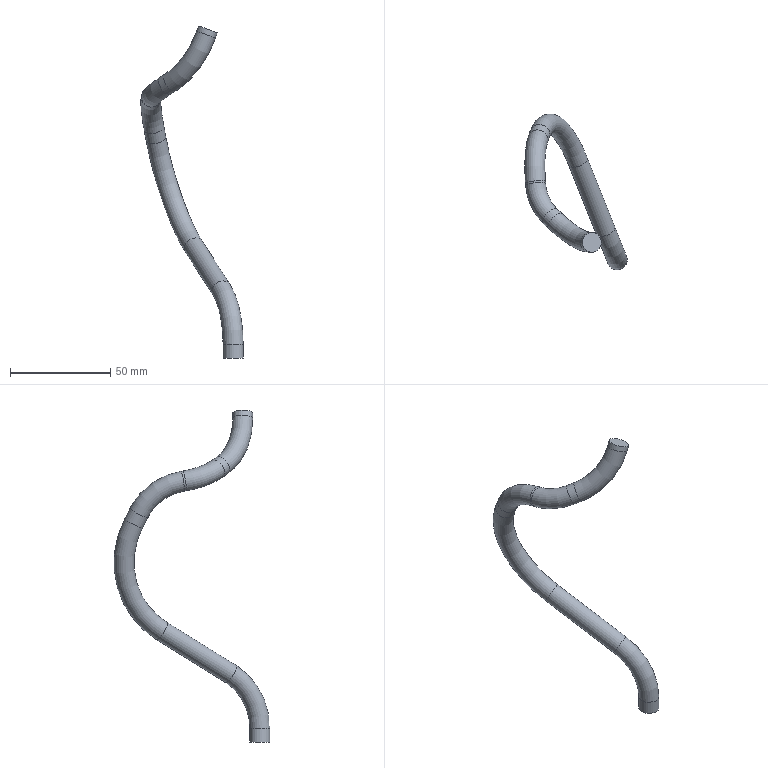Part | STEP file | DEWALT-DWE7294-B3-03 | 1 solid | 13 faces | box 51.027 x 77.706 x 165.503 mm | volume 18773 mm3 | cylinder 6 | torus 5 | plane 2 | commonest cylinder face diameters 10 x6
STEP:
#1=CARTESIAN_POINT('',(0.,0.,0.));
#2=DIRECTION('',(0.,0.,1.));
#3=DIRECTION('',(1.,0.,0.));
#4=AXIS2_PLACEMENT_3D('',#1,#2,#3);
#5=CARTESIAN_POINT('',(5.,0.,0.));
#6=VERTEX_POINT('',#5);
#7=CARTESIAN_POINT('',(0.,0.,0.));
#8=DIRECTION('',(0.,0.,-1.));
#9=DIRECTION('',(1.,0.,0.));
#10=AXIS2_PLACEMENT_3D('',#7,#8,#9);
#11=CIRCLE('',#10,5.);
#12=CARTESIAN_POINT('',(0.,0.,6.811));
#13=DIRECTION('',(0.,0.,-1.));
#14=DIRECTION('',(-1.,0.,0.));
#15=AXIS2_PLACEMENT_3D('',#12,#13,#14);
#16=CYLINDRICAL_SURFACE('',#15,5.);
#17=CARTESIAN_POINT('',(3.142,6.811));
#18=DIRECTION('',(1.,0.));
#19=VECTOR('',#18,1.);
#20=LINE('',#17,#19);
#21=(GEOMETRIC_REPRESENTATION_CONTEXT(2)PARAMETRIC_REPRESENTATION_CONTEXT()REPRESENTATION_CONTEXT('',''));
#22=DEFINITIONAL_REPRESENTATION('',(#20),#21);
#23=PCURVE('',#16,#22);
#24=CARTESIAN_POINT('',(0.,0.,0.));
#25=DIRECTION('',(0.,0.,-1.));
#26=DIRECTION('',(-1.,0.,0.));
#27=AXIS2_PLACEMENT_3D('',#24,#25,#26);
#28=PLANE('',#27);
#29=CARTESIAN_POINT('',(0.,0.));
#30=DIRECTION('',(-1.,0.));
#31=AXIS2_PLACEMENT_2D('',#29,#30);
#32=CIRCLE('',#31,5.);
#33=(GEOMETRIC_REPRESENTATION_CONTEXT(2)PARAMETRIC_REPRESENTATION_CONTEXT()REPRESENTATION_CONTEXT('',''));
#34=DEFINITIONAL_REPRESENTATION('',(#32),#33);
#35=PCURVE('',#28,#34);
#36=SURFACE_CURVE('',#11,(#23,#35),.PCURVE_S1.);
#37=EDGE_CURVE('',#6,#6,#36,.T.);
#38=ORIENTED_EDGE('',*,*,#37,.F.);
#39=CARTESIAN_POINT('',(5.,0.,6.811));
#40=VERTEX_POINT('',#39);
#41=CARTESIAN_POINT('',(5.,0.,6.811));
#42=CARTESIAN_POINT('',(5.,0.,0.));
#43=B_SPLINE_CURVE_WITH_KNOTS('',1,(#41,#42),.UNSPECIFIED.,.F.,.F.,(2,2),(0.,6.811),.PIECEWISE_BEZIER_KNOTS.);
#44=CARTESIAN_POINT('',(3.142,0.));
#45=DIRECTION('',(0.,1.));
#46=VECTOR('',#45,1.);
#47=LINE('',#44,#46);
#48=(GEOMETRIC_REPRESENTATION_CONTEXT(2)PARAMETRIC_REPRESENTATION_CONTEXT()REPRESENTATION_CONTEXT('',''));
#49=DEFINITIONAL_REPRESENTATION('',(#47),#48);
#50=PCURVE('',#16,#49);
#51=CARTESIAN_POINT('',(9.425,0.));
#52=DIRECTION('',(0.,1.));
#53=VECTOR('',#52,1.);
#54=LINE('',#51,#53);
#55=(GEOMETRIC_REPRESENTATION_CONTEXT(2)PARAMETRIC_REPRESENTATION_CONTEXT()REPRESENTATION_CONTEXT('',''));
#56=DEFINITIONAL_REPRESENTATION('',(#54),#55);
#57=PCURVE('',#16,#56);
#58=SEAM_CURVE('',#43,(#50,#57),.PCURVE_S1.);
#59=EDGE_CURVE('',#40,#6,#58,.T.);
#60=ORIENTED_EDGE('',*,*,#59,.F.);
#61=CARTESIAN_POINT('',(0.,0.,6.811));
#62=DIRECTION('',(0.,0.,-1.));
#63=DIRECTION('',(1.,0.,0.));
#64=AXIS2_PLACEMENT_3D('',#61,#62,#63);
#65=CIRCLE('',#64,5.);
#66=CARTESIAN_POINT('',(3.142,0.));
#67=DIRECTION('',(1.,0.));
#68=VECTOR('',#67,1.);
#69=LINE('',#66,#68);
#70=(GEOMETRIC_REPRESENTATION_CONTEXT(2)PARAMETRIC_REPRESENTATION_CONTEXT()REPRESENTATION_CONTEXT('',''));
#71=DEFINITIONAL_REPRESENTATION('',(#69),#70);
#72=PCURVE('',#16,#71);
#73=CARTESIAN_POINT('',(-11.672,29.262,6.811));
#74=DIRECTION('',(0.9288,0.3705,0.));
#75=DIRECTION('',(-0.3705,0.9288,0.));
#76=AXIS2_PLACEMENT_3D('',#73,#74,#75);
#77=TOROIDAL_SURFACE('',#76,31.504,5.);
#78=CARTESIAN_POINT('',(3.142,7.474));
#79=DIRECTION('',(0.,-1.));
#80=VECTOR('',#79,1.);
#81=LINE('',#78,#80);
#82=(GEOMETRIC_REPRESENTATION_CONTEXT(2)PARAMETRIC_REPRESENTATION_CONTEXT()REPRESENTATION_CONTEXT('',''));
#83=DEFINITIONAL_REPRESENTATION('',(#81),#82);
#84=PCURVE('',#77,#83);
#85=SURFACE_CURVE('',#65,(#72,#84),.PCURVE_S1.);
#86=EDGE_CURVE('',#40,#40,#85,.T.);
#87=ORIENTED_EDGE('',*,*,#86,.T.);
#88=ORIENTED_EDGE('',*,*,#59,.T.);
#89=EDGE_LOOP('',(#38,#60,#87,#88));
#90=FACE_BOUND('',#89,.T.);
#91=ADVANCED_FACE('',(#90),#16,.T.);
#92=ORIENTED_EDGE('',*,*,#86,.F.);
#93=CARTESIAN_POINT('',(-1.179,15.491,35.699));
#94=VERTEX_POINT('',#93);
#95=CARTESIAN_POINT('',(-1.179,15.491,35.699));
#96=CARTESIAN_POINT('',(0.706,10.765,32.761));
#97=CARTESIAN_POINT('',(2.341,6.666,28.785));
#98=CARTESIAN_POINT('',(3.641,3.406,23.952));
#99=CARTESIAN_POINT('',(4.542,1.149,18.496));
#100=CARTESIAN_POINT('',(5.,0.,12.687));
#101=CARTESIAN_POINT('',(5.,0.,6.811));
#102=(BOUNDED_CURVE()B_SPLINE_CURVE(6,(#95,#96,#97,#98,#99,#100,#101),.UNSPECIFIED.,.F.,.F.)B_SPLINE_CURVE_WITH_KNOTS((7,7),(2.094,3.142),.PIECEWISE_BEZIER_KNOTS.)CURVE()GEOMETRIC_REPRESENTATION_ITEM()RATIONAL_B_SPLINE_CURVE((1.014,1.005,0.9991,0.9973,0.9991,1.005,1.014))REPRESENTATION_ITEM(''));
#103=CARTESIAN_POINT('',(0.,7.474));
#104=DIRECTION('',(1.,0.));
#105=VECTOR('',#104,1.);
#106=LINE('',#103,#105);
#107=(GEOMETRIC_REPRESENTATION_CONTEXT(2)PARAMETRIC_REPRESENTATION_CONTEXT()REPRESENTATION_CONTEXT('',''));
#108=DEFINITIONAL_REPRESENTATION('',(#106),#107);
#109=PCURVE('',#77,#108);
#110=CARTESIAN_POINT('',(0.,1.191));
#111=DIRECTION('',(1.,0.));
#112=VECTOR('',#111,1.);
#113=LINE('',#110,#112);
#114=(GEOMETRIC_REPRESENTATION_CONTEXT(2)PARAMETRIC_REPRESENTATION_CONTEXT()REPRESENTATION_CONTEXT('',''));
#115=DEFINITIONAL_REPRESENTATION('',(#113),#114);
#116=PCURVE('',#77,#115);
#117=SEAM_CURVE('',#102,(#109,#116),.PCURVE_S1.);
#118=EDGE_CURVE('',#94,#40,#117,.T.);
#119=ORIENTED_EDGE('',*,*,#118,.F.);
#120=CARTESIAN_POINT('',(-5.836,14.631,34.094));
#121=DIRECTION('',(0.3209,-0.8044,-0.5));
#122=DIRECTION('',(0.9314,0.1721,0.3209));
#123=AXIS2_PLACEMENT_3D('',#120,#121,#122);
#124=CIRCLE('',#123,5.);
#125=CARTESIAN_POINT('',(2.094,7.474));
#126=DIRECTION('',(0.,-1.));
#127=VECTOR('',#126,1.);
#128=LINE('',#125,#127);
#129=(GEOMETRIC_REPRESENTATION_CONTEXT(2)PARAMETRIC_REPRESENTATION_CONTEXT()REPRESENTATION_CONTEXT('',''));
#130=DEFINITIONAL_REPRESENTATION('',(#128),#129);
#131=PCURVE('',#77,#130);
#132=CARTESIAN_POINT('',(-19.569,49.06,55.495));
#133=DIRECTION('',(0.3209,-0.8044,-0.5));
#134=DIRECTION('',(0.,0.5279,-0.8493));
#135=AXIS2_PLACEMENT_3D('',#132,#133,#134);
#136=CYLINDRICAL_SURFACE('',#135,5.);
#137=CARTESIAN_POINT('',(1.753,42.801));
#138=DIRECTION('',(1.,0.));
#139=VECTOR('',#138,1.);
#140=LINE('',#137,#139);
#141=(GEOMETRIC_REPRESENTATION_CONTEXT(2)PARAMETRIC_REPRESENTATION_CONTEXT()REPRESENTATION_CONTEXT('',''));
#142=DEFINITIONAL_REPRESENTATION('',(#140),#141);
#143=PCURVE('',#136,#142);
#144=SURFACE_CURVE('',#124,(#131,#143),.PCURVE_S1.);
#145=EDGE_CURVE('',#94,#94,#144,.T.);
#146=ORIENTED_EDGE('',*,*,#145,.T.);
#147=ORIENTED_EDGE('',*,*,#118,.T.);
#148=EDGE_LOOP('',(#92,#119,#146,#147));
#149=FACE_BOUND('',#148,.T.);
#150=ADVANCED_FACE('',(#149),#77,.T.);
#151=ORIENTED_EDGE('',*,*,#145,.F.);
#152=CARTESIAN_POINT('',(-14.913,49.92,57.099));
#153=VERTEX_POINT('',#152);
#154=CARTESIAN_POINT('',(-14.913,49.92,57.099));
#155=CARTESIAN_POINT('',(-1.179,15.491,35.699));
#156=B_SPLINE_CURVE_WITH_KNOTS('',1,(#154,#155),.UNSPECIFIED.,.F.,.F.,(2,2),(0.,42.801),.PIECEWISE_BEZIER_KNOTS.);
#157=CARTESIAN_POINT('',(1.753,0.));
#158=DIRECTION('',(0.,1.));
#159=VECTOR('',#158,1.);
#160=LINE('',#157,#159);
#161=(GEOMETRIC_REPRESENTATION_CONTEXT(2)PARAMETRIC_REPRESENTATION_CONTEXT()REPRESENTATION_CONTEXT('',''));
#162=DEFINITIONAL_REPRESENTATION('',(#160),#161);
#163=PCURVE('',#136,#162);
#164=CARTESIAN_POINT('',(8.037,0.));
#165=DIRECTION('',(0.,1.));
#166=VECTOR('',#165,1.);
#167=LINE('',#164,#166);
#168=(GEOMETRIC_REPRESENTATION_CONTEXT(2)PARAMETRIC_REPRESENTATION_CONTEXT()REPRESENTATION_CONTEXT('',''));
#169=DEFINITIONAL_REPRESENTATION('',(#167),#168);
#170=PCURVE('',#136,#169);
#171=SEAM_CURVE('',#156,(#163,#170),.PCURVE_S1.);
#172=EDGE_CURVE('',#153,#94,#171,.T.);
#173=ORIENTED_EDGE('',*,*,#172,.F.);
#174=CARTESIAN_POINT('',(-19.569,49.06,55.495));
#175=DIRECTION('',(0.3209,-0.8044,-0.5));
#176=DIRECTION('',(0.9314,0.1721,0.3209));
#177=AXIS2_PLACEMENT_3D('',#174,#175,#176);
#178=CIRCLE('',#177,5.);
#179=CARTESIAN_POINT('',(1.753,0.));
#180=DIRECTION('',(1.,0.));
#181=VECTOR('',#180,1.);
#182=LINE('',#179,#181);
#183=(GEOMETRIC_REPRESENTATION_CONTEXT(2)PARAMETRIC_REPRESENTATION_CONTEXT()REPRESENTATION_CONTEXT('',''));
#184=DEFINITIONAL_REPRESENTATION('',(#182),#183);
#185=PCURVE('',#136,#184);
#186=CARTESIAN_POINT('',(-25.022,24.287,91.849));
#187=DIRECTION('',(-0.9391,-0.2016,-0.2783));
#188=DIRECTION('',(-0.2841,0.,0.9588));
#189=AXIS2_PLACEMENT_3D('',#186,#187,#188);
#190=TOROIDAL_SURFACE('',#189,44.329,5.);
#191=CARTESIAN_POINT('',(2.534,4.66));
#192=DIRECTION('',(0.,-1.));
#193=VECTOR('',#192,1.);
#194=LINE('',#191,#193);
#195=(GEOMETRIC_REPRESENTATION_CONTEXT(2)PARAMETRIC_REPRESENTATION_CONTEXT()REPRESENTATION_CONTEXT('',''));
#196=DEFINITIONAL_REPRESENTATION('',(#194),#195);
#197=PCURVE('',#190,#196);
#198=SURFACE_CURVE('',#178,(#185,#197),.PCURVE_S1.);
#199=EDGE_CURVE('',#153,#153,#198,.T.);
#200=ORIENTED_EDGE('',*,*,#199,.T.);
#201=ORIENTED_EDGE('',*,*,#172,.T.);
#202=EDGE_LOOP('',(#151,#173,#200,#201));
#203=FACE_BOUND('',#202,.T.);
#204=ADVANCED_FACE('',(#203),#136,.T.);
#205=ORIENTED_EDGE('',*,*,#199,.F.);
#206=CARTESIAN_POINT('',(-33.669,63.584,110.499));
#207=VERTEX_POINT('',#206);
#208=CARTESIAN_POINT('',(-33.669,63.584,110.499));
#209=CARTESIAN_POINT('',(-31.912,68.461,101.037));
#210=CARTESIAN_POINT('',(-29.242,70.498,90.549));
#211=CARTESIAN_POINT('',(-25.886,69.431,79.995));
#212=CARTESIAN_POINT('',(-22.148,65.33,70.351));
#213=CARTESIAN_POINT('',(-18.374,58.599,62.494));
#214=CARTESIAN_POINT('',(-14.913,49.92,57.099));
#215=(BOUNDED_CURVE()B_SPLINE_CURVE(6,(#208,#209,#210,#211,#212,#213,#214),.UNSPECIFIED.,.F.,.F.)B_SPLINE_CURVE_WITH_KNOTS((7,7),(1.091,2.534),.PIECEWISE_BEZIER_KNOTS.)CURVE()GEOMETRIC_REPRESENTATION_ITEM()RATIONAL_B_SPLINE_CURVE((1.026,1.008,0.9982,0.9949,0.9982,1.008,1.026))REPRESENTATION_ITEM(''));
#216=CARTESIAN_POINT('',(0.,4.66));
#217=DIRECTION('',(1.,0.));
#218=VECTOR('',#217,1.);
#219=LINE('',#216,#218);
#220=(GEOMETRIC_REPRESENTATION_CONTEXT(2)PARAMETRIC_REPRESENTATION_CONTEXT()REPRESENTATION_CONTEXT('',''));
#221=DEFINITIONAL_REPRESENTATION('',(#219),#220);
#222=PCURVE('',#190,#221);
#223=CARTESIAN_POINT('',(0.,-1.623));
#224=DIRECTION('',(1.,0.));
#225=VECTOR('',#224,1.);
#226=LINE('',#223,#225);
#227=(GEOMETRIC_REPRESENTATION_CONTEXT(2)PARAMETRIC_REPRESENTATION_CONTEXT()REPRESENTATION_CONTEXT('',''));
#228=DEFINITIONAL_REPRESENTATION('',(#226),#227);
#229=PCURVE('',#190,#228);
#230=SEAM_CURVE('',#215,(#222,#229),.PCURVE_S1.);
#231=EDGE_CURVE('',#207,#153,#230,.T.);
#232=ORIENTED_EDGE('',*,*,#231,.F.);
#233=CARTESIAN_POINT('',(-38.437,62.805,109.213));
#234=DIRECTION('',(0.1628,0.452,-0.877));
#235=DIRECTION('',(0.9537,0.1558,0.2573));
#236=AXIS2_PLACEMENT_3D('',#233,#234,#235);
#237=CIRCLE('',#236,5.);
#238=CARTESIAN_POINT('',(1.091,4.66));
#239=DIRECTION('',(0.,-1.));
#240=VECTOR('',#239,1.);
#241=LINE('',#238,#240);
#242=(GEOMETRIC_REPRESENTATION_CONTEXT(2)PARAMETRIC_REPRESENTATION_CONTEXT()REPRESENTATION_CONTEXT('',''));
#243=DEFINITIONAL_REPRESENTATION('',(#241),#242);
#244=PCURVE('',#190,#243);
#245=CARTESIAN_POINT('',(-39.385,60.173,114.32));
#246=DIRECTION('',(0.1628,0.452,-0.877));
#247=DIRECTION('',(0.,0.8889,0.4582));
#248=AXIS2_PLACEMENT_3D('',#245,#246,#247);
#249=CYLINDRICAL_SURFACE('',#248,5.);
#250=CARTESIAN_POINT('',(1.312,5.823));
#251=DIRECTION('',(1.,0.));
#252=VECTOR('',#251,1.);
#253=LINE('',#250,#252);
#254=(GEOMETRIC_REPRESENTATION_CONTEXT(2)PARAMETRIC_REPRESENTATION_CONTEXT()REPRESENTATION_CONTEXT('',''));
#255=DEFINITIONAL_REPRESENTATION('',(#253),#254);
#256=PCURVE('',#249,#255);
#257=SURFACE_CURVE('',#237,(#244,#256),.PCURVE_S1.);
#258=EDGE_CURVE('',#207,#207,#257,.T.);
#259=ORIENTED_EDGE('',*,*,#258,.T.);
#260=ORIENTED_EDGE('',*,*,#231,.T.);
#261=EDGE_LOOP('',(#205,#232,#259,#260));
#262=FACE_BOUND('',#261,.T.);
#263=ADVANCED_FACE('',(#262),#190,.T.);
#264=ORIENTED_EDGE('',*,*,#258,.F.);
#265=CARTESIAN_POINT('',(-34.617,60.952,115.606));
#266=VERTEX_POINT('',#265);
#267=CARTESIAN_POINT('',(-34.617,60.952,115.606));
#268=CARTESIAN_POINT('',(-33.669,63.584,110.499));
#269=B_SPLINE_CURVE_WITH_KNOTS('',1,(#267,#268),.UNSPECIFIED.,.F.,.F.,(2,2),(0.,5.823),.PIECEWISE_BEZIER_KNOTS.);
#270=CARTESIAN_POINT('',(1.312,0.));
#271=DIRECTION('',(0.,1.));
#272=VECTOR('',#271,1.);
#273=LINE('',#270,#272);
#274=(GEOMETRIC_REPRESENTATION_CONTEXT(2)PARAMETRIC_REPRESENTATION_CONTEXT()REPRESENTATION_CONTEXT('',''));
#275=DEFINITIONAL_REPRESENTATION('',(#273),#274);
#276=PCURVE('',#249,#275);
#277=CARTESIAN_POINT('',(7.595,0.));
#278=DIRECTION('',(0.,1.));
#279=VECTOR('',#278,1.);
#280=LINE('',#277,#279);
#281=(GEOMETRIC_REPRESENTATION_CONTEXT(2)PARAMETRIC_REPRESENTATION_CONTEXT()REPRESENTATION_CONTEXT('',''));
#282=DEFINITIONAL_REPRESENTATION('',(#280),#281);
#283=PCURVE('',#249,#282);
#284=SEAM_CURVE('',#269,(#276,#283),.PCURVE_S1.);
#285=EDGE_CURVE('',#266,#207,#284,.T.);
#286=ORIENTED_EDGE('',*,*,#285,.F.);
#287=CARTESIAN_POINT('',(-39.385,60.173,114.32));
#288=DIRECTION('',(0.1628,0.452,-0.877));
#289=DIRECTION('',(0.9537,0.1558,0.2573));
#290=AXIS2_PLACEMENT_3D('',#287,#288,#289);
#291=CIRCLE('',#290,5.);
#292=CARTESIAN_POINT('',(1.312,0.));
#293=DIRECTION('',(1.,0.));
#294=VECTOR('',#293,1.);
#295=LINE('',#292,#294);
#296=(GEOMETRIC_REPRESENTATION_CONTEXT(2)PARAMETRIC_REPRESENTATION_CONTEXT()REPRESENTATION_CONTEXT('',''));
#297=DEFINITIONAL_REPRESENTATION('',(#295),#296);
#298=PCURVE('',#249,#297);
#299=CARTESIAN_POINT('',(-33.388,34.461,102.18));
#300=DIRECTION('',(-0.9648,-0.113,-0.2373));
#301=DIRECTION('',(-0.2389,0.,0.9711));
#302=AXIS2_PLACEMENT_3D('',#299,#300,#301);
#303=TOROIDAL_SURFACE('',#302,29.059,5.);
#304=CARTESIAN_POINT('',(1.098,4.761));
#305=DIRECTION('',(0.,-1.));
#306=VECTOR('',#305,1.);
#307=LINE('',#304,#306);
#308=(GEOMETRIC_REPRESENTATION_CONTEXT(2)PARAMETRIC_REPRESENTATION_CONTEXT()REPRESENTATION_CONTEXT('',''));
#309=DEFINITIONAL_REPRESENTATION('',(#307),#308);
#310=PCURVE('',#303,#309);
#311=SURFACE_CURVE('',#291,(#298,#310),.PCURVE_S1.);
#312=EDGE_CURVE('',#266,#266,#311,.T.);
#313=ORIENTED_EDGE('',*,*,#312,.T.);
#314=ORIENTED_EDGE('',*,*,#285,.T.);
#315=EDGE_LOOP('',(#264,#286,#313,#314));
#316=FACE_BOUND('',#315,.T.);
#317=ADVANCED_FACE('',(#316),#249,.T.);
#318=ORIENTED_EDGE('',*,*,#312,.F.);
#319=CARTESIAN_POINT('',(-35.941,38.984,131.447));
#320=VERTEX_POINT('',#319);
#321=CARTESIAN_POINT('',(-35.941,38.984,131.447));
#322=CARTESIAN_POINT('',(-36.302,43.645,130.695));
#323=CARTESIAN_POINT('',(-36.429,48.139,129.073));
#324=CARTESIAN_POINT('',(-36.315,52.275,126.639));
#325=CARTESIAN_POINT('',(-35.962,55.881,123.49));
#326=CARTESIAN_POINT('',(-35.388,58.811,119.759));
#327=CARTESIAN_POINT('',(-34.617,60.952,115.606));
#328=(BOUNDED_CURVE()B_SPLINE_CURVE(6,(#321,#322,#323,#324,#325,#326,#327),.UNSPECIFIED.,.F.,.F.)B_SPLINE_CURVE_WITH_KNOTS((7,7),(0.1364,1.098),.PIECEWISE_BEZIER_KNOTS.)CURVE()GEOMETRIC_REPRESENTATION_ITEM()RATIONAL_B_SPLINE_CURVE((1.012,1.004,0.9992,0.9977,0.9992,1.004,1.012))REPRESENTATION_ITEM(''));
#329=CARTESIAN_POINT('',(0.,4.761));
#330=DIRECTION('',(1.,0.));
#331=VECTOR('',#330,1.);
#332=LINE('',#329,#331);
#333=(GEOMETRIC_REPRESENTATION_CONTEXT(2)PARAMETRIC_REPRESENTATION_CONTEXT()REPRESENTATION_CONTEXT('',''));
#334=DEFINITIONAL_REPRESENTATION('',(#332),#333);
#335=PCURVE('',#303,#334);
#336=CARTESIAN_POINT('',(0.,-1.522));
#337=DIRECTION('',(1.,0.));
#338=VECTOR('',#337,1.);
#339=LINE('',#336,#338);
#340=(GEOMETRIC_REPRESENTATION_CONTEXT(2)PARAMETRIC_REPRESENTATION_CONTEXT()REPRESENTATION_CONTEXT('',''));
#341=DEFINITIONAL_REPRESENTATION('',(#339),#340);
#342=PCURVE('',#303,#341);
#343=SEAM_CURVE('',#328,(#335,#342),.PCURVE_S1.);
#344=EDGE_CURVE('',#320,#266,#343,.T.);
#345=ORIENTED_EDGE('',*,*,#344,.F.);
#346=CARTESIAN_POINT('',(-40.698,38.387,130.029));
#347=DIRECTION('',(-0.0762,0.9844,-0.1588));
#348=DIRECTION('',(0.9515,0.1194,0.2836));
#349=AXIS2_PLACEMENT_3D('',#346,#347,#348);
#350=CIRCLE('',#349,5.);
#351=CARTESIAN_POINT('',(0.1364,4.761));
#352=DIRECTION('',(0.,-1.));
#353=VECTOR('',#352,1.);
#354=LINE('',#351,#353);
#355=(GEOMETRIC_REPRESENTATION_CONTEXT(2)PARAMETRIC_REPRESENTATION_CONTEXT()REPRESENTATION_CONTEXT('',''));
#356=DEFINITIONAL_REPRESENTATION('',(#354),#355);
#357=PCURVE('',#303,#356);
#358=CARTESIAN_POINT('',(-40.622,37.403,130.188));
#359=DIRECTION('',(-0.0762,0.9844,-0.1588));
#360=DIRECTION('',(0.,0.1593,0.9872));
#361=AXIS2_PLACEMENT_3D('',#358,#359,#360);
#362=CYLINDRICAL_SURFACE('',#361,5.);
#363=CARTESIAN_POINT('',(1.267,1.));
#364=DIRECTION('',(1.,0.));
#365=VECTOR('',#364,1.);
#366=LINE('',#363,#365);
#367=(GEOMETRIC_REPRESENTATION_CONTEXT(2)PARAMETRIC_REPRESENTATION_CONTEXT()REPRESENTATION_CONTEXT('',''));
#368=DEFINITIONAL_REPRESENTATION('',(#366),#367);
#369=PCURVE('',#362,#368);
#370=SURFACE_CURVE('',#350,(#357,#369),.PCURVE_S1.);
#371=EDGE_CURVE('',#320,#320,#370,.T.);
#372=ORIENTED_EDGE('',*,*,#371,.T.);
#373=ORIENTED_EDGE('',*,*,#344,.T.);
#374=EDGE_LOOP('',(#318,#345,#372,#373));
#375=FACE_BOUND('',#374,.T.);
#376=ADVANCED_FACE('',(#375),#303,.T.);
#377=ORIENTED_EDGE('',*,*,#371,.F.);
#378=CARTESIAN_POINT('',(-35.865,38.,131.606));
#379=VERTEX_POINT('',#378);
#380=CARTESIAN_POINT('',(-35.865,38.,131.606));
#381=CARTESIAN_POINT('',(-35.941,38.984,131.447));
#382=B_SPLINE_CURVE_WITH_KNOTS('',1,(#380,#381),.UNSPECIFIED.,.F.,.F.,(2,2),(0.,1.),.PIECEWISE_BEZIER_KNOTS.);
#383=CARTESIAN_POINT('',(1.267,0.));
#384=DIRECTION('',(0.,1.));
#385=VECTOR('',#384,1.);
#386=LINE('',#383,#385);
#387=(GEOMETRIC_REPRESENTATION_CONTEXT(2)PARAMETRIC_REPRESENTATION_CONTEXT()REPRESENTATION_CONTEXT('',''));
#388=DEFINITIONAL_REPRESENTATION('',(#386),#387);
#389=PCURVE('',#362,#388);
#390=CARTESIAN_POINT('',(7.55,0.));
#391=DIRECTION('',(0.,1.));
#392=VECTOR('',#391,1.);
#393=LINE('',#390,#392);
#394=(GEOMETRIC_REPRESENTATION_CONTEXT(2)PARAMETRIC_REPRESENTATION_CONTEXT()REPRESENTATION_CONTEXT('',''));
#395=DEFINITIONAL_REPRESENTATION('',(#393),#394);
#396=PCURVE('',#362,#395);
#397=SEAM_CURVE('',#382,(#389,#396),.PCURVE_S1.);
#398=EDGE_CURVE('',#379,#320,#397,.T.);
#399=ORIENTED_EDGE('',*,*,#398,.F.);
#400=CARTESIAN_POINT('',(-40.622,37.403,130.188));
#401=DIRECTION('',(-0.0762,0.9844,-0.1588));
#402=DIRECTION('',(0.9515,0.1194,0.2836));
#403=AXIS2_PLACEMENT_3D('',#400,#401,#402);
#404=CIRCLE('',#403,5.);
#405=CARTESIAN_POINT('',(1.267,0.));
#406=DIRECTION('',(1.,0.));
#407=VECTOR('',#406,1.);
#408=LINE('',#405,#407);
#409=(GEOMETRIC_REPRESENTATION_CONTEXT(2)PARAMETRIC_REPRESENTATION_CONTEXT()REPRESENTATION_CONTEXT('',''));
#410=DEFINITIONAL_REPRESENTATION('',(#408),#409);
#411=PCURVE('',#362,#410);
#412=CARTESIAN_POINT('',(-18.618,40.934,141.516));
#413=DIRECTION('',(0.4685,-0.1052,-0.8772));
#414=DIRECTION('',(-0.8821,0.,-0.4711));
#415=AXIS2_PLACEMENT_3D('',#412,#413,#414);
#416=TOROIDAL_SURFACE('',#415,25.,5.);
#417=CARTESIAN_POINT('',(6.141,9.239));
#418=DIRECTION('',(0.,-1.));
#419=VECTOR('',#418,1.);
#420=LINE('',#417,#419);
#421=(GEOMETRIC_REPRESENTATION_CONTEXT(2)PARAMETRIC_REPRESENTATION_CONTEXT()REPRESENTATION_CONTEXT('',''));
#422=DEFINITIONAL_REPRESENTATION('',(#420),#421);
#423=PCURVE('',#416,#422);
#424=SURFACE_CURVE('',#404,(#411,#423),.PCURVE_S1.);
#425=EDGE_CURVE('',#379,#379,#424,.T.);
#426=ORIENTED_EDGE('',*,*,#425,.T.);
#427=ORIENTED_EDGE('',*,*,#398,.T.);
#428=EDGE_LOOP('',(#377,#399,#426,#427));
#429=FACE_BOUND('',#428,.T.);
#430=ADVANCED_FACE('',(#429),#362,.T.);
#431=ORIENTED_EDGE('',*,*,#425,.F.);
#432=CARTESIAN_POINT('',(-30.031,25.239,136.253));
#433=VERTEX_POINT('',#432);
#434=CARTESIAN_POINT('',(-30.031,25.239,136.253));
#435=CARTESIAN_POINT('',(-31.698,26.814,135.174));
#436=CARTESIAN_POINT('',(-33.13,28.677,134.185));
#437=CARTESIAN_POINT('',(-34.288,30.782,133.314));
#438=CARTESIAN_POINT('',(-35.142,33.078,132.582));
#439=CARTESIAN_POINT('',(-35.672,35.505,132.009));
#440=CARTESIAN_POINT('',(-35.865,38.,131.606));
#441=(BOUNDED_CURVE()B_SPLINE_CURVE(6,(#434,#435,#436,#437,#438,#439,#440),.UNSPECIFIED.,.F.,.F.)B_SPLINE_CURVE_WITH_KNOTS((7,7),(5.387,6.141),.PIECEWISE_BEZIER_KNOTS.)CURVE()GEOMETRIC_REPRESENTATION_ITEM()RATIONAL_B_SPLINE_CURVE((1.007,1.002,0.9995,0.9986,0.9995,1.002,1.007))REPRESENTATION_ITEM(''));
#442=CARTESIAN_POINT('',(0.,9.239));
#443=DIRECTION('',(1.,0.));
#444=VECTOR('',#443,1.);
#445=LINE('',#442,#444);
#446=(GEOMETRIC_REPRESENTATION_CONTEXT(2)PARAMETRIC_REPRESENTATION_CONTEXT()REPRESENTATION_CONTEXT('',''));
#447=DEFINITIONAL_REPRESENTATION('',(#445),#446);
#448=PCURVE('',#416,#447);
#449=CARTESIAN_POINT('',(0.,2.956));
#450=DIRECTION('',(1.,0.));
#451=VECTOR('',#450,1.);
#452=LINE('',#449,#451);
#453=(GEOMETRIC_REPRESENTATION_CONTEXT(2)PARAMETRIC_REPRESENTATION_CONTEXT()REPRESENTATION_CONTEXT('',''));
#454=DEFINITIONAL_REPRESENTATION('',(#452),#453);
#455=PCURVE('',#416,#454);
#456=SEAM_CURVE('',#441,(#448,#455),.PCURVE_S1.);
#457=EDGE_CURVE('',#433,#379,#456,.T.);
#458=ORIENTED_EDGE('',*,*,#457,.F.);
#459=CARTESIAN_POINT('',(-33.361,21.52,135.972));
#460=DIRECTION('',(-0.6578,0.6212,-0.4259));
#461=DIRECTION('',(0.666,0.7438,0.05621));
#462=AXIS2_PLACEMENT_3D('',#459,#460,#461);
#463=CIRCLE('',#462,5.);
#464=CARTESIAN_POINT('',(5.387,9.239));
#465=DIRECTION('',(0.,-1.));
#466=VECTOR('',#465,1.);
#467=LINE('',#464,#466);
#468=(GEOMETRIC_REPRESENTATION_CONTEXT(2)PARAMETRIC_REPRESENTATION_CONTEXT()REPRESENTATION_CONTEXT('',''));
#469=DEFINITIONAL_REPRESENTATION('',(#467),#468);
#470=PCURVE('',#416,#469);
#471=CARTESIAN_POINT('',(-30.758,19.062,137.657));
#472=DIRECTION('',(-0.6578,0.6212,-0.4259));
#473=DIRECTION('',(-0.6866,-0.7271,0.));
#474=AXIS2_PLACEMENT_3D('',#471,#472,#473);
#475=CYLINDRICAL_SURFACE('',#474,5.);
#476=CARTESIAN_POINT('',(3.079,3.956));
#477=DIRECTION('',(1.,0.));
#478=VECTOR('',#477,1.);
#479=LINE('',#476,#478);
#480=(GEOMETRIC_REPRESENTATION_CONTEXT(2)PARAMETRIC_REPRESENTATION_CONTEXT()REPRESENTATION_CONTEXT('',''));
#481=DEFINITIONAL_REPRESENTATION('',(#479),#480);
#482=PCURVE('',#475,#481);
#483=SURFACE_CURVE('',#463,(#470,#482),.PCURVE_S1.);
#484=EDGE_CURVE('',#433,#433,#483,.T.);
#485=ORIENTED_EDGE('',*,*,#484,.T.);
#486=ORIENTED_EDGE('',*,*,#457,.T.);
#487=EDGE_LOOP('',(#431,#458,#485,#486));
#488=FACE_BOUND('',#487,.T.);
#489=ADVANCED_FACE('',(#488),#416,.T.);
#490=ORIENTED_EDGE('',*,*,#484,.F.);
#491=CARTESIAN_POINT('',(-27.428,22.781,137.938));
#492=VERTEX_POINT('',#491);
#493=CARTESIAN_POINT('',(-27.428,22.781,137.938));
#494=CARTESIAN_POINT('',(-30.031,25.239,136.253));
#495=B_SPLINE_CURVE_WITH_KNOTS('',1,(#493,#494),.UNSPECIFIED.,.F.,.F.,(2,2),(0.,3.956),.PIECEWISE_BEZIER_KNOTS.);
#496=CARTESIAN_POINT('',(3.079,0.));
#497=DIRECTION('',(0.,1.));
#498=VECTOR('',#497,1.);
#499=LINE('',#496,#498);
#500=(GEOMETRIC_REPRESENTATION_CONTEXT(2)PARAMETRIC_REPRESENTATION_CONTEXT()REPRESENTATION_CONTEXT('',''));
#501=DEFINITIONAL_REPRESENTATION('',(#499),#500);
#502=PCURVE('',#475,#501);
#503=CARTESIAN_POINT('',(9.363,0.));
#504=DIRECTION('',(0.,1.));
#505=VECTOR('',#504,1.);
#506=LINE('',#503,#505);
#507=(GEOMETRIC_REPRESENTATION_CONTEXT(2)PARAMETRIC_REPRESENTATION_CONTEXT()REPRESENTATION_CONTEXT('',''));
#508=DEFINITIONAL_REPRESENTATION('',(#506),#507);
#509=PCURVE('',#475,#508);
#510=SEAM_CURVE('',#495,(#502,#509),.PCURVE_S1.);
#511=EDGE_CURVE('',#492,#433,#510,.T.);
#512=ORIENTED_EDGE('',*,*,#511,.F.);
#513=CARTESIAN_POINT('',(-30.758,19.062,137.657));
#514=DIRECTION('',(-0.6578,0.6212,-0.4259));
#515=DIRECTION('',(0.666,0.7438,0.05621));
#516=AXIS2_PLACEMENT_3D('',#513,#514,#515);
#517=CIRCLE('',#516,5.);
#518=CARTESIAN_POINT('',(3.079,0.));
#519=DIRECTION('',(1.,0.));
#520=VECTOR('',#519,1.);
#521=LINE('',#518,#520);
#522=(GEOMETRIC_REPRESENTATION_CONTEXT(2)PARAMETRIC_REPRESENTATION_CONTEXT()REPRESENTATION_CONTEXT('',''));
#523=DEFINITIONAL_REPRESENTATION('',(#521),#522);
#524=PCURVE('',#475,#523);
#525=CARTESIAN_POINT('',(-33.736,36.913,168.295));
#526=DIRECTION('',(0.7485,0.6021,-0.278));
#527=DIRECTION('',(-0.6268,0.7792,0.));
#528=AXIS2_PLACEMENT_3D('',#525,#526,#527);
#529=TOROIDAL_SURFACE('',#528,35.584,5.);
#530=CARTESIAN_POINT('',(4.253,8.228));
#531=DIRECTION('',(0.,-1.));
#532=VECTOR('',#531,1.);
#533=LINE('',#530,#532);
#534=(GEOMETRIC_REPRESENTATION_CONTEXT(2)PARAMETRIC_REPRESENTATION_CONTEXT()REPRESENTATION_CONTEXT('',''));
#535=DEFINITIONAL_REPRESENTATION('',(#533),#534);
#536=PCURVE('',#529,#535);
#537=SURFACE_CURVE('',#517,(#524,#536),.PCURVE_S1.);
#538=EDGE_CURVE('',#492,#492,#537,.T.);
#539=ORIENTED_EDGE('',*,*,#538,.T.);
#540=ORIENTED_EDGE('',*,*,#511,.T.);
#541=EDGE_LOOP('',(#490,#512,#539,#540));
#542=FACE_BOUND('',#541,.T.);
#543=ADVANCED_FACE('',(#542),#475,.T.);
#544=ORIENTED_EDGE('',*,*,#538,.F.);
#545=CARTESIAN_POINT('',(-11.075,12.764,160.271));
#546=VERTEX_POINT('',#545);
#547=CARTESIAN_POINT('',(-11.075,12.764,160.271));
#548=CARTESIAN_POINT('',(-12.823,12.72,155.468));
#549=CARTESIAN_POINT('',(-15.083,13.415,150.89));
#550=CARTESIAN_POINT('',(-17.777,14.832,146.706));
#551=CARTESIAN_POINT('',(-20.808,16.922,143.071));
#552=CARTESIAN_POINT('',(-24.065,19.606,140.115));
#553=CARTESIAN_POINT('',(-27.428,22.781,137.938));
#554=(BOUNDED_CURVE()B_SPLINE_CURVE(6,(#547,#548,#549,#550,#551,#552,#553),.UNSPECIFIED.,.F.,.F.)B_SPLINE_CURVE_WITH_KNOTS((7,7),(3.351,4.253),.PIECEWISE_BEZIER_KNOTS.)CURVE()GEOMETRIC_REPRESENTATION_ITEM()RATIONAL_B_SPLINE_CURVE((1.01,1.003,0.9993,0.998,0.9993,1.003,1.01))REPRESENTATION_ITEM(''));
#555=CARTESIAN_POINT('',(0.,8.228));
#556=DIRECTION('',(1.,0.));
#557=VECTOR('',#556,1.);
#558=LINE('',#555,#557);
#559=(GEOMETRIC_REPRESENTATION_CONTEXT(2)PARAMETRIC_REPRESENTATION_CONTEXT()REPRESENTATION_CONTEXT('',''));
#560=DEFINITIONAL_REPRESENTATION('',(#558),#559);
#561=PCURVE('',#529,#560);
#562=CARTESIAN_POINT('',(0.,1.945));
#563=DIRECTION('',(1.,0.));
#564=VECTOR('',#563,1.);
#565=LINE('',#562,#564);
#566=(GEOMETRIC_REPRESENTATION_CONTEXT(2)PARAMETRIC_REPRESENTATION_CONTEXT()REPRESENTATION_CONTEXT('',''));
#567=DEFINITIONAL_REPRESENTATION('',(#565),#566);
#568=PCURVE('',#529,#567);
#569=SEAM_CURVE('',#554,(#561,#568),.PCURVE_S1.);
#570=EDGE_CURVE('',#546,#492,#569,.T.);
#571=ORIENTED_EDGE('',*,*,#570,.F.);
#572=CARTESIAN_POINT('',(-13.519,8.502,161.2));
#573=DIRECTION('',(-0.342,-0.008727,-0.9397));
#574=DIRECTION('',(0.4888,0.8524,-0.1858));
#575=AXIS2_PLACEMENT_3D('',#572,#573,#574);
#576=CIRCLE('',#575,5.);
#577=CARTESIAN_POINT('',(3.351,8.228));
#578=DIRECTION('',(0.,-1.));
#579=VECTOR('',#578,1.);
#580=LINE('',#577,#579);
#581=(GEOMETRIC_REPRESENTATION_CONTEXT(2)PARAMETRIC_REPRESENTATION_CONTEXT()REPRESENTATION_CONTEXT('',''));
#582=DEFINITIONAL_REPRESENTATION('',(#580),#581);
#583=PCURVE('',#529,#582);
#584=CARTESIAN_POINT('',(-12.576,8.527,163.793));
#585=DIRECTION('',(-0.342,-0.008727,-0.9397));
#586=DIRECTION('',(-0.9397,0.,0.342));
#587=AXIS2_PLACEMENT_3D('',#584,#585,#586);
#588=CYLINDRICAL_SURFACE('',#587,5.);
#589=CARTESIAN_POINT('',(2.121,2.759));
#590=DIRECTION('',(1.,0.));
#591=VECTOR('',#590,1.);
#592=LINE('',#589,#591);
#593=(GEOMETRIC_REPRESENTATION_CONTEXT(2)PARAMETRIC_REPRESENTATION_CONTEXT()REPRESENTATION_CONTEXT('',''));
#594=DEFINITIONAL_REPRESENTATION('',(#592),#593);
#595=PCURVE('',#588,#594);
#596=SURFACE_CURVE('',#576,(#583,#595),.PCURVE_S1.);
#597=EDGE_CURVE('',#546,#546,#596,.T.);
#598=ORIENTED_EDGE('',*,*,#597,.T.);
#599=ORIENTED_EDGE('',*,*,#570,.T.);
#600=EDGE_LOOP('',(#544,#571,#598,#599));
#601=FACE_BOUND('',#600,.T.);
#602=ADVANCED_FACE('',(#601),#529,.T.);
#603=ORIENTED_EDGE('',*,*,#597,.F.);
#604=CARTESIAN_POINT('',(-10.132,12.788,162.863));
#605=VERTEX_POINT('',#604);
#606=CARTESIAN_POINT('',(-10.132,12.788,162.863));
#607=CARTESIAN_POINT('',(-11.075,12.764,160.271));
#608=B_SPLINE_CURVE_WITH_KNOTS('',1,(#606,#607),.UNSPECIFIED.,.F.,.F.,(2,2),(0.,2.759),.PIECEWISE_BEZIER_KNOTS.);
#609=CARTESIAN_POINT('',(2.121,0.));
#610=DIRECTION('',(0.,1.));
#611=VECTOR('',#610,1.);
#612=LINE('',#609,#611);
#613=(GEOMETRIC_REPRESENTATION_CONTEXT(2)PARAMETRIC_REPRESENTATION_CONTEXT()REPRESENTATION_CONTEXT('',''));
#614=DEFINITIONAL_REPRESENTATION('',(#612),#613);
#615=PCURVE('',#588,#614);
#616=CARTESIAN_POINT('',(8.404,0.));
#617=DIRECTION('',(0.,1.));
#618=VECTOR('',#617,1.);
#619=LINE('',#616,#618);
#620=(GEOMETRIC_REPRESENTATION_CONTEXT(2)PARAMETRIC_REPRESENTATION_CONTEXT()REPRESENTATION_CONTEXT('',''));
#621=DEFINITIONAL_REPRESENTATION('',(#619),#620);
#622=PCURVE('',#588,#621);
#623=SEAM_CURVE('',#608,(#615,#622),.PCURVE_S1.);
#624=EDGE_CURVE('',#605,#546,#623,.T.);
#625=ORIENTED_EDGE('',*,*,#624,.F.);
#626=CARTESIAN_POINT('',(-12.576,8.527,163.793));
#627=DIRECTION('',(-0.342,-0.008727,-0.9397));
#628=DIRECTION('',(0.4888,0.8524,-0.1858));
#629=AXIS2_PLACEMENT_3D('',#626,#627,#628);
#630=CIRCLE('',#629,5.);
#631=CARTESIAN_POINT('',(2.121,0.));
#632=DIRECTION('',(1.,0.));
#633=VECTOR('',#632,1.);
#634=LINE('',#631,#633);
#635=(GEOMETRIC_REPRESENTATION_CONTEXT(2)PARAMETRIC_REPRESENTATION_CONTEXT()REPRESENTATION_CONTEXT('',''));
#636=DEFINITIONAL_REPRESENTATION('',(#634),#635);
#637=PCURVE('',#588,#636);
#638=CARTESIAN_POINT('',(-12.576,8.527,163.793));
#639=DIRECTION('',(-0.342,-0.008727,-0.9397));
#640=DIRECTION('',(-0.4888,-0.8524,0.1858));
#641=AXIS2_PLACEMENT_3D('',#638,#639,#640);
#642=PLANE('',#641);
#643=CARTESIAN_POINT('',(0.,0.));
#644=DIRECTION('',(-1.,0.));
#645=AXIS2_PLACEMENT_2D('',#643,#644);
#646=CIRCLE('',#645,5.);
#647=(GEOMETRIC_REPRESENTATION_CONTEXT(2)PARAMETRIC_REPRESENTATION_CONTEXT()REPRESENTATION_CONTEXT('',''));
#648=DEFINITIONAL_REPRESENTATION('',(#646),#647);
#649=PCURVE('',#642,#648);
#650=SURFACE_CURVE('',#630,(#637,#649),.PCURVE_S1.);
#651=EDGE_CURVE('',#605,#605,#650,.T.);
#652=ORIENTED_EDGE('',*,*,#651,.T.);
#653=ORIENTED_EDGE('',*,*,#624,.T.);
#654=EDGE_LOOP('',(#603,#625,#652,#653));
#655=FACE_BOUND('',#654,.T.);
#656=ADVANCED_FACE('',(#655),#588,.T.);
#657=ORIENTED_EDGE('',*,*,#37,.T.);
#658=EDGE_LOOP('',(#657));
#659=FACE_BOUND('',#658,.T.);
#660=ADVANCED_FACE('',(#659),#28,.T.);
#661=ORIENTED_EDGE('',*,*,#651,.F.);
#662=EDGE_LOOP('',(#661));
#663=FACE_BOUND('',#662,.T.);
#664=ADVANCED_FACE('',(#663),#642,.F.);
#665=CLOSED_SHELL('',(#91,#150,#204,#263,#317,#376,#430,#489,#543,#602,#656,#660,#664));
#666=MANIFOLD_SOLID_BREP('',#665);
#667=(LENGTH_UNIT()NAMED_UNIT(*)SI_UNIT(.MILLI.,.METRE.));
#668=UNCERTAINTY_MEASURE_WITH_UNIT(LENGTH_MEASURE(0.000001),#667,'','');
#669=(NAMED_UNIT(*)PLANE_ANGLE_UNIT()SI_UNIT($,.RADIAN.));
#670=(NAMED_UNIT(*)SI_UNIT($,.STERADIAN.)SOLID_ANGLE_UNIT());
#671=(GEOMETRIC_REPRESENTATION_CONTEXT(3)GLOBAL_UNCERTAINTY_ASSIGNED_CONTEXT((#668))GLOBAL_UNIT_ASSIGNED_CONTEXT((#667,#669,#670))REPRESENTATION_CONTEXT('',''));
#672=ADVANCED_BREP_SHAPE_REPRESENTATION('',(#4,#666),#671);